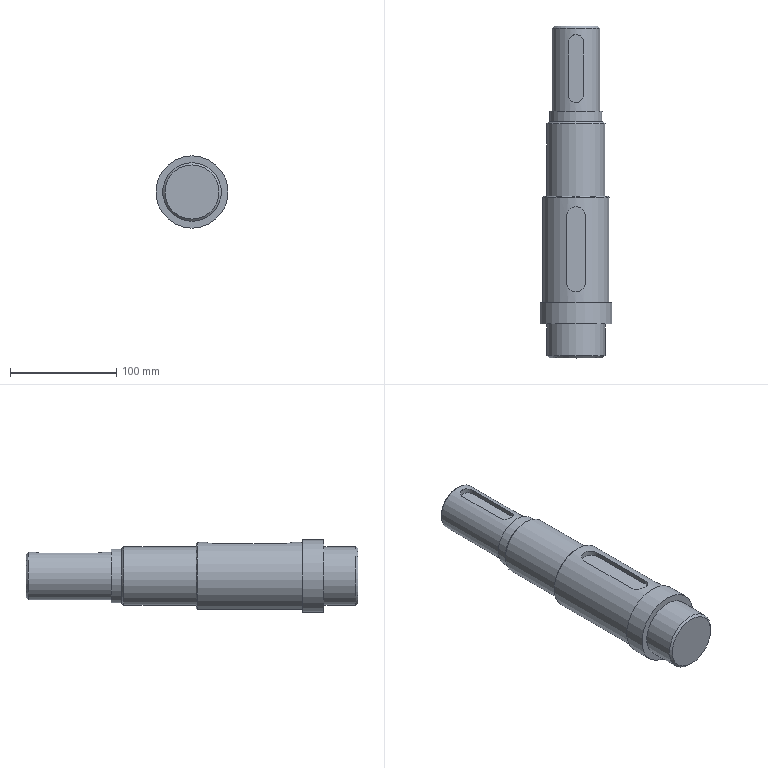Part | NX | features DATUM_CSYS 4, CHAMFER 3, SKETCH 3, DATUM_PLANE 2, EXTRUDE 2, SWP104 1 | 1 solid | 27 faces | box 68 x 312 x 68 mm | volume 761578 mm3 | plane 13 | cylinder 10 | cone 4 | commonest cylinder face diameters 14 x2 18 x2 55 x2 45 x1 50 x1 63 x1
STEP:
#1=CARTESIAN_POINT('',(0.,310.,22.5));
#2=VERTEX_POINT('',#1);
#3=CARTESIAN_POINT('',(0.,310.,0.));
#4=DIRECTION('',(0.,1.,0.));
#5=DIRECTION('',(0.,0.,1.));
#6=AXIS2_PLACEMENT_3D('',#3,#4,#5);
#7=CIRCLE('',#6,22.5);
#8=EDGE_CURVE('',#2,#2,#7,.F.);
#9=ORIENTED_EDGE('',*,*,#8,.T.);
#10=EDGE_LOOP('',(#9));
#11=FACE_BOUND('',#10,.T.);
#12=CARTESIAN_POINT('',(0.,232.,22.5));
#13=VERTEX_POINT('',#12);
#14=CARTESIAN_POINT('',(0.,232.,0.));
#15=DIRECTION('',(0.,1.,0.));
#16=DIRECTION('',(0.,0.,1.));
#17=AXIS2_PLACEMENT_3D('',#14,#15,#16);
#18=CIRCLE('',#17,22.5);
#19=EDGE_CURVE('',#13,#13,#18,.T.);
#20=ORIENTED_EDGE('',*,*,#19,.T.);
#21=EDGE_LOOP('',(#20));
#22=FACE_BOUND('',#21,.T.);
#23=CARTESIAN_POINT('',(7.,297.,21.383));
#24=VERTEX_POINT('',#23);
#25=CARTESIAN_POINT('',(7.,247.,21.383));
#26=VERTEX_POINT('',#25);
#27=CARTESIAN_POINT('',(7.,0.,21.383));
#28=DIRECTION('',(0.,1.,0.));
#29=VECTOR('',#28,1000.);
#30=LINE('',#27,#29);
#31=EDGE_CURVE('',#24,#26,#30,.F.);
#32=ORIENTED_EDGE('',*,*,#31,.T.);
#33=CARTESIAN_POINT('',(-7.,247.,21.383));
#34=VERTEX_POINT('',#33);
#35=CARTESIAN_POINT('',(7.,247.,21.383));
#36=CARTESIAN_POINT('',(7.,245.138,21.383));
#37=CARTESIAN_POINT('',(5.483,241.532,21.956));
#38=CARTESIAN_POINT('',(0.01146,239.235,22.772));
#39=CARTESIAN_POINT('',(-5.486,241.529,21.957));
#40=CARTESIAN_POINT('',(-7.,245.138,21.383));
#41=CARTESIAN_POINT('',(-7.,247.,21.383));
#42=B_SPLINE_CURVE_WITH_KNOTS('',3,(#35,#36,#37,#38,#39,#40,#41),.UNSPECIFIED.,.F.,.F.,(4,1,1,1,4),(0.,0.005504,0.01101,0.01651,0.02201),.UNSPECIFIED.);
#43=EDGE_CURVE('',#26,#34,#42,.T.);
#44=ORIENTED_EDGE('',*,*,#43,.T.);
#45=CARTESIAN_POINT('',(-7.,297.,21.383));
#46=VERTEX_POINT('',#45);
#47=CARTESIAN_POINT('',(-7.,0.,21.383));
#48=DIRECTION('',(0.,1.,0.));
#49=VECTOR('',#48,1000.);
#50=LINE('',#47,#49);
#51=EDGE_CURVE('',#34,#46,#50,.T.);
#52=ORIENTED_EDGE('',*,*,#51,.T.);
#53=CARTESIAN_POINT('',(-7.,297.,21.383));
#54=CARTESIAN_POINT('',(-7.,298.862,21.383));
#55=CARTESIAN_POINT('',(-5.483,302.468,21.956));
#56=CARTESIAN_POINT('',(-0.01146,304.765,22.772));
#57=CARTESIAN_POINT('',(5.486,302.471,21.957));
#58=CARTESIAN_POINT('',(7.,298.862,21.383));
#59=CARTESIAN_POINT('',(7.,297.,21.383));
#60=B_SPLINE_CURVE_WITH_KNOTS('',3,(#53,#54,#55,#56,#57,#58,#59),.UNSPECIFIED.,.F.,.F.,(4,1,1,1,4),(0.,0.005504,0.01101,0.01651,0.02201),.UNSPECIFIED.);
#61=EDGE_CURVE('',#46,#24,#60,.T.);
#62=ORIENTED_EDGE('',*,*,#61,.T.);
#63=EDGE_LOOP('',(#32,#44,#52,#62));
#64=FACE_BOUND('',#63,.T.);
#65=CARTESIAN_POINT('',(0.,0.,0.));
#66=DIRECTION('',(0.,1.,0.));
#67=DIRECTION('',(0.,0.,1.));
#68=AXIS2_PLACEMENT_3D('',#65,#66,#67);
#69=CYLINDRICAL_SURFACE('',#68,22.5);
#70=ADVANCED_FACE('',(#11,#22,#64),#69,.T.);
#71=CARTESIAN_POINT('',(0.,151.,31.5));
#72=VERTEX_POINT('',#71);
#73=CARTESIAN_POINT('',(0.,151.,0.));
#74=DIRECTION('',(0.,1.,0.));
#75=DIRECTION('',(0.,0.,1.));
#76=AXIS2_PLACEMENT_3D('',#73,#74,#75);
#77=CIRCLE('',#76,31.5);
#78=EDGE_CURVE('',#72,#72,#77,.F.);
#79=ORIENTED_EDGE('',*,*,#78,.T.);
#80=EDGE_LOOP('',(#79));
#81=FACE_BOUND('',#80,.T.);
#82=CARTESIAN_POINT('',(0.,52.,31.5));
#83=VERTEX_POINT('',#82);
#84=CARTESIAN_POINT('',(0.,52.,0.));
#85=DIRECTION('',(0.,1.,0.));
#86=DIRECTION('',(0.,0.,1.));
#87=AXIS2_PLACEMENT_3D('',#84,#85,#86);
#88=CIRCLE('',#87,31.5);
#89=EDGE_CURVE('',#83,#83,#88,.T.);
#90=ORIENTED_EDGE('',*,*,#89,.T.);
#91=EDGE_LOOP('',(#90));
#92=FACE_BOUND('',#91,.T.);
#93=CARTESIAN_POINT('',(9.,133.,30.187));
#94=VERTEX_POINT('',#93);
#95=CARTESIAN_POINT('',(9.,71.,30.187));
#96=VERTEX_POINT('',#95);
#97=CARTESIAN_POINT('',(9.,0.,30.187));
#98=DIRECTION('',(0.,1.,0.));
#99=VECTOR('',#98,1000.);
#100=LINE('',#97,#99);
#101=EDGE_CURVE('',#94,#96,#100,.F.);
#102=ORIENTED_EDGE('',*,*,#101,.T.);
#103=CARTESIAN_POINT('',(-9.,71.,30.187));
#104=VERTEX_POINT('',#103);
#105=CARTESIAN_POINT('',(9.,71.,30.187));
#106=CARTESIAN_POINT('',(9.,68.609,30.187));
#107=CARTESIAN_POINT('',(7.049,63.968,30.857));
#108=CARTESIAN_POINT('',(0.01381,61.017,31.821));
#109=CARTESIAN_POINT('',(-7.053,63.964,30.858));
#110=CARTESIAN_POINT('',(-9.,68.609,30.187));
#111=CARTESIAN_POINT('',(-9.,71.,30.187));
#112=B_SPLINE_CURVE_WITH_KNOTS('',3,(#105,#106,#107,#108,#109,#110,#111),.UNSPECIFIED.,.F.,.F.,(4,1,1,1,4),(0.,0.007069,0.01414,0.02121,0.02828),.UNSPECIFIED.);
#113=EDGE_CURVE('',#96,#104,#112,.T.);
#114=ORIENTED_EDGE('',*,*,#113,.T.);
#115=CARTESIAN_POINT('',(-9.,133.,30.187));
#116=VERTEX_POINT('',#115);
#117=CARTESIAN_POINT('',(-9.,0.,30.187));
#118=DIRECTION('',(0.,1.,0.));
#119=VECTOR('',#118,1000.);
#120=LINE('',#117,#119);
#121=EDGE_CURVE('',#104,#116,#120,.T.);
#122=ORIENTED_EDGE('',*,*,#121,.T.);
#123=CARTESIAN_POINT('',(-9.,133.,30.187));
#124=CARTESIAN_POINT('',(-9.,135.391,30.187));
#125=CARTESIAN_POINT('',(-7.049,140.032,30.857));
#126=CARTESIAN_POINT('',(-0.01381,142.983,31.821));
#127=CARTESIAN_POINT('',(7.053,140.036,30.858));
#128=CARTESIAN_POINT('',(9.,135.391,30.187));
#129=CARTESIAN_POINT('',(9.,133.,30.187));
#130=B_SPLINE_CURVE_WITH_KNOTS('',3,(#123,#124,#125,#126,#127,#128,#129),.UNSPECIFIED.,.F.,.F.,(4,1,1,1,4),(0.,0.007069,0.01414,0.02121,0.02828),.UNSPECIFIED.);
#131=EDGE_CURVE('',#116,#94,#130,.T.);
#132=ORIENTED_EDGE('',*,*,#131,.T.);
#133=EDGE_LOOP('',(#102,#114,#122,#132));
#134=FACE_BOUND('',#133,.T.);
#135=CARTESIAN_POINT('',(0.,0.,0.));
#136=DIRECTION('',(0.,1.,0.));
#137=DIRECTION('',(0.,0.,1.));
#138=AXIS2_PLACEMENT_3D('',#135,#136,#137);
#139=CYLINDRICAL_SURFACE('',#138,31.5);
#140=ADVANCED_FACE('',(#81,#92,#134),#139,.T.);
#141=CARTESIAN_POINT('',(0.,312.,20.5));
#142=VERTEX_POINT('',#141);
#143=CARTESIAN_POINT('',(0.,312.,0.));
#144=DIRECTION('',(0.,1.,0.));
#145=DIRECTION('',(0.,0.,1.));
#146=AXIS2_PLACEMENT_3D('',#143,#144,#145);
#147=CIRCLE('',#146,20.5);
#148=EDGE_CURVE('',#142,#142,#147,.T.);
#149=ORIENTED_EDGE('',*,*,#148,.T.);
#150=EDGE_LOOP('',(#149));
#151=FACE_BOUND('',#150,.T.);
#152=CARTESIAN_POINT('',(0.,312.,0.));
#153=DIRECTION('',(0.,1.,0.));
#154=DIRECTION('',(0.,0.,1.));
#155=AXIS2_PLACEMENT_3D('',#152,#153,#154);
#156=PLANE('',#155);
#157=ADVANCED_FACE('',(#151),#156,.T.);
#158=CARTESIAN_POINT('',(0.,232.,25.));
#159=VERTEX_POINT('',#158);
#160=CARTESIAN_POINT('',(0.,232.,0.));
#161=DIRECTION('',(0.,1.,0.));
#162=DIRECTION('',(0.,0.,1.));
#163=AXIS2_PLACEMENT_3D('',#160,#161,#162);
#164=CIRCLE('',#163,25.);
#165=EDGE_CURVE('',#159,#159,#164,.T.);
#166=ORIENTED_EDGE('',*,*,#165,.T.);
#167=EDGE_LOOP('',(#166));
#168=FACE_BOUND('',#167,.T.);
#169=ORIENTED_EDGE('',*,*,#19,.F.);
#170=EDGE_LOOP('',(#169));
#171=FACE_BOUND('',#170,.T.);
#172=CARTESIAN_POINT('',(0.,232.,22.5));
#173=DIRECTION('',(0.,1.,0.));
#174=DIRECTION('',(0.,0.,1.));
#175=AXIS2_PLACEMENT_3D('',#172,#173,#174);
#176=PLANE('',#175);
#177=ADVANCED_FACE('',(#168,#171),#176,.T.);
#178=CARTESIAN_POINT('',(0.,222.,25.));
#179=VERTEX_POINT('',#178);
#180=CARTESIAN_POINT('',(0.,222.,0.));
#181=DIRECTION('',(0.,1.,0.));
#182=DIRECTION('',(0.,0.,1.));
#183=AXIS2_PLACEMENT_3D('',#180,#181,#182);
#184=CIRCLE('',#183,25.);
#185=EDGE_CURVE('',#179,#179,#184,.T.);
#186=ORIENTED_EDGE('',*,*,#185,.T.);
#187=EDGE_LOOP('',(#186));
#188=FACE_BOUND('',#187,.T.);
#189=ORIENTED_EDGE('',*,*,#165,.F.);
#190=EDGE_LOOP('',(#189));
#191=FACE_BOUND('',#190,.T.);
#192=CARTESIAN_POINT('',(0.,0.,0.));
#193=DIRECTION('',(0.,1.,0.));
#194=DIRECTION('',(0.,0.,1.));
#195=AXIS2_PLACEMENT_3D('',#192,#193,#194);
#196=CYLINDRICAL_SURFACE('',#195,25.);
#197=ADVANCED_FACE('',(#188,#191),#196,.T.);
#198=CARTESIAN_POINT('',(0.,222.,25.5));
#199=VERTEX_POINT('',#198);
#200=CARTESIAN_POINT('',(0.,222.,0.));
#201=DIRECTION('',(0.,1.,0.));
#202=DIRECTION('',(0.,0.,1.));
#203=AXIS2_PLACEMENT_3D('',#200,#201,#202);
#204=CIRCLE('',#203,25.5);
#205=EDGE_CURVE('',#199,#199,#204,.T.);
#206=ORIENTED_EDGE('',*,*,#205,.T.);
#207=EDGE_LOOP('',(#206));
#208=FACE_BOUND('',#207,.T.);
#209=ORIENTED_EDGE('',*,*,#185,.F.);
#210=EDGE_LOOP('',(#209));
#211=FACE_BOUND('',#210,.T.);
#212=CARTESIAN_POINT('',(0.,222.,25.));
#213=DIRECTION('',(0.,1.,0.));
#214=DIRECTION('',(0.,0.,1.));
#215=AXIS2_PLACEMENT_3D('',#212,#213,#214);
#216=PLANE('',#215);
#217=ADVANCED_FACE('',(#208,#211),#216,.T.);
#218=CARTESIAN_POINT('',(0.,220.,27.5));
#219=VERTEX_POINT('',#218);
#220=CARTESIAN_POINT('',(0.,220.,0.));
#221=DIRECTION('',(0.,1.,0.));
#222=DIRECTION('',(0.,0.,1.));
#223=AXIS2_PLACEMENT_3D('',#220,#221,#222);
#224=CIRCLE('',#223,27.5);
#225=EDGE_CURVE('',#219,#219,#224,.F.);
#226=ORIENTED_EDGE('',*,*,#225,.T.);
#227=EDGE_LOOP('',(#226));
#228=FACE_BOUND('',#227,.T.);
#229=CARTESIAN_POINT('',(0.,152.,27.5));
#230=VERTEX_POINT('',#229);
#231=CARTESIAN_POINT('',(0.,152.,0.));
#232=DIRECTION('',(0.,1.,0.));
#233=DIRECTION('',(0.,0.,1.));
#234=AXIS2_PLACEMENT_3D('',#231,#232,#233);
#235=CIRCLE('',#234,27.5);
#236=EDGE_CURVE('',#230,#230,#235,.T.);
#237=ORIENTED_EDGE('',*,*,#236,.T.);
#238=EDGE_LOOP('',(#237));
#239=FACE_BOUND('',#238,.T.);
#240=CARTESIAN_POINT('',(0.,0.,0.));
#241=DIRECTION('',(0.,1.,0.));
#242=DIRECTION('',(0.,0.,1.));
#243=AXIS2_PLACEMENT_3D('',#240,#241,#242);
#244=CYLINDRICAL_SURFACE('',#243,27.5);
#245=ADVANCED_FACE('',(#228,#239),#244,.T.);
#246=CARTESIAN_POINT('',(0.,152.,30.5));
#247=VERTEX_POINT('',#246);
#248=CARTESIAN_POINT('',(0.,152.,0.));
#249=DIRECTION('',(0.,1.,0.));
#250=DIRECTION('',(0.,0.,1.));
#251=AXIS2_PLACEMENT_3D('',#248,#249,#250);
#252=CIRCLE('',#251,30.5);
#253=EDGE_CURVE('',#247,#247,#252,.T.);
#254=ORIENTED_EDGE('',*,*,#253,.T.);
#255=EDGE_LOOP('',(#254));
#256=FACE_BOUND('',#255,.T.);
#257=ORIENTED_EDGE('',*,*,#236,.F.);
#258=EDGE_LOOP('',(#257));
#259=FACE_BOUND('',#258,.T.);
#260=CARTESIAN_POINT('',(0.,152.,27.5));
#261=DIRECTION('',(0.,1.,0.));
#262=DIRECTION('',(0.,0.,1.));
#263=AXIS2_PLACEMENT_3D('',#260,#261,#262);
#264=PLANE('',#263);
#265=ADVANCED_FACE('',(#256,#259),#264,.T.);
#266=CARTESIAN_POINT('',(0.,52.,34.));
#267=VERTEX_POINT('',#266);
#268=CARTESIAN_POINT('',(0.,52.,0.));
#269=DIRECTION('',(0.,1.,0.));
#270=DIRECTION('',(0.,0.,1.));
#271=AXIS2_PLACEMENT_3D('',#268,#269,#270);
#272=CIRCLE('',#271,34.);
#273=EDGE_CURVE('',#267,#267,#272,.T.);
#274=ORIENTED_EDGE('',*,*,#273,.T.);
#275=EDGE_LOOP('',(#274));
#276=FACE_BOUND('',#275,.T.);
#277=ORIENTED_EDGE('',*,*,#89,.F.);
#278=EDGE_LOOP('',(#277));
#279=FACE_BOUND('',#278,.T.);
#280=CARTESIAN_POINT('',(0.,52.,31.5));
#281=DIRECTION('',(0.,1.,0.));
#282=DIRECTION('',(0.,0.,1.));
#283=AXIS2_PLACEMENT_3D('',#280,#281,#282);
#284=PLANE('',#283);
#285=ADVANCED_FACE('',(#276,#279),#284,.T.);
#286=CARTESIAN_POINT('',(0.,32.,34.));
#287=VERTEX_POINT('',#286);
#288=CARTESIAN_POINT('',(0.,32.,0.));
#289=DIRECTION('',(0.,1.,0.));
#290=DIRECTION('',(0.,0.,1.));
#291=AXIS2_PLACEMENT_3D('',#288,#289,#290);
#292=CIRCLE('',#291,34.);
#293=EDGE_CURVE('',#287,#287,#292,.T.);
#294=ORIENTED_EDGE('',*,*,#293,.T.);
#295=EDGE_LOOP('',(#294));
#296=FACE_BOUND('',#295,.T.);
#297=ORIENTED_EDGE('',*,*,#273,.F.);
#298=EDGE_LOOP('',(#297));
#299=FACE_BOUND('',#298,.T.);
#300=CARTESIAN_POINT('',(0.,0.,0.));
#301=DIRECTION('',(0.,1.,0.));
#302=DIRECTION('',(0.,0.,1.));
#303=AXIS2_PLACEMENT_3D('',#300,#301,#302);
#304=CYLINDRICAL_SURFACE('',#303,34.);
#305=ADVANCED_FACE('',(#296,#299),#304,.T.);
#306=CARTESIAN_POINT('',(0.,32.,27.5));
#307=VERTEX_POINT('',#306);
#308=CARTESIAN_POINT('',(0.,32.,0.));
#309=DIRECTION('',(0.,1.,0.));
#310=DIRECTION('',(0.,0.,1.));
#311=AXIS2_PLACEMENT_3D('',#308,#309,#310);
#312=CIRCLE('',#311,27.5);
#313=EDGE_CURVE('',#307,#307,#312,.T.);
#314=ORIENTED_EDGE('',*,*,#313,.T.);
#315=EDGE_LOOP('',(#314));
#316=FACE_BOUND('',#315,.T.);
#317=ORIENTED_EDGE('',*,*,#293,.F.);
#318=EDGE_LOOP('',(#317));
#319=FACE_BOUND('',#318,.T.);
#320=CARTESIAN_POINT('',(0.,32.,34.));
#321=DIRECTION('',(0.,-1.,0.));
#322=DIRECTION('',(0.,0.,-1.));
#323=AXIS2_PLACEMENT_3D('',#320,#321,#322);
#324=PLANE('',#323);
#325=ADVANCED_FACE('',(#316,#319),#324,.T.);
#326=CARTESIAN_POINT('',(0.,2.,-27.5));
#327=VERTEX_POINT('',#326);
#328=CARTESIAN_POINT('',(0.,2.,0.));
#329=DIRECTION('',(0.,-1.,0.));
#330=DIRECTION('',(0.,0.,-1.));
#331=AXIS2_PLACEMENT_3D('',#328,#329,#330);
#332=CIRCLE('',#331,27.5);
#333=EDGE_CURVE('',#327,#327,#332,.F.);
#334=ORIENTED_EDGE('',*,*,#333,.T.);
#335=EDGE_LOOP('',(#334));
#336=FACE_BOUND('',#335,.T.);
#337=ORIENTED_EDGE('',*,*,#313,.F.);
#338=EDGE_LOOP('',(#337));
#339=FACE_BOUND('',#338,.T.);
#340=CARTESIAN_POINT('',(0.,0.,0.));
#341=DIRECTION('',(0.,1.,0.));
#342=DIRECTION('',(0.,0.,1.));
#343=AXIS2_PLACEMENT_3D('',#340,#341,#342);
#344=CYLINDRICAL_SURFACE('',#343,27.5);
#345=ADVANCED_FACE('',(#336,#339),#344,.T.);
#346=CARTESIAN_POINT('',(0.,0.,-25.5));
#347=VERTEX_POINT('',#346);
#348=CARTESIAN_POINT('',(0.,0.,0.));
#349=DIRECTION('',(0.,-1.,0.));
#350=DIRECTION('',(0.,0.,-1.));
#351=AXIS2_PLACEMENT_3D('',#348,#349,#350);
#352=CIRCLE('',#351,25.5);
#353=EDGE_CURVE('',#347,#347,#352,.T.);
#354=ORIENTED_EDGE('',*,*,#353,.T.);
#355=EDGE_LOOP('',(#354));
#356=FACE_BOUND('',#355,.T.);
#357=CARTESIAN_POINT('',(0.,0.,27.5));
#358=DIRECTION('',(0.,-1.,0.));
#359=DIRECTION('',(0.,0.,-1.));
#360=AXIS2_PLACEMENT_3D('',#357,#358,#359);
#361=PLANE('',#360);
#362=ADVANCED_FACE('',(#356),#361,.T.);
#363=ORIENTED_EDGE('',*,*,#8,.F.);
#364=EDGE_LOOP('',(#363));
#365=FACE_BOUND('',#364,.T.);
#366=ORIENTED_EDGE('',*,*,#148,.F.);
#367=EDGE_LOOP('',(#366));
#368=FACE_BOUND('',#367,.T.);
#369=CARTESIAN_POINT('',(0.,312.,0.));
#370=DIRECTION('',(0.,-1.,0.));
#371=DIRECTION('',(0.,0.,-1.));
#372=AXIS2_PLACEMENT_3D('',#369,#370,#371);
#373=CONICAL_SURFACE('',#372,20.5,0.7854);
#374=ADVANCED_FACE('',(#365,#368),#373,.T.);
#375=ORIENTED_EDGE('',*,*,#353,.F.);
#376=EDGE_LOOP('',(#375));
#377=FACE_BOUND('',#376,.T.);
#378=ORIENTED_EDGE('',*,*,#333,.F.);
#379=EDGE_LOOP('',(#378));
#380=FACE_BOUND('',#379,.T.);
#381=CARTESIAN_POINT('',(0.,2.,0.));
#382=DIRECTION('',(0.,1.,0.));
#383=DIRECTION('',(0.,0.,1.));
#384=AXIS2_PLACEMENT_3D('',#381,#382,#383);
#385=CONICAL_SURFACE('',#384,27.5,0.7854);
#386=ADVANCED_FACE('',(#377,#380),#385,.T.);
#387=ORIENTED_EDGE('',*,*,#78,.F.);
#388=EDGE_LOOP('',(#387));
#389=FACE_BOUND('',#388,.T.);
#390=ORIENTED_EDGE('',*,*,#253,.F.);
#391=EDGE_LOOP('',(#390));
#392=FACE_BOUND('',#391,.T.);
#393=CARTESIAN_POINT('',(0.,152.,0.));
#394=DIRECTION('',(0.,-1.,0.));
#395=DIRECTION('',(0.,0.,-1.));
#396=AXIS2_PLACEMENT_3D('',#393,#394,#395);
#397=CONICAL_SURFACE('',#396,30.5,0.7854);
#398=ADVANCED_FACE('',(#389,#392),#397,.T.);
#399=CARTESIAN_POINT('',(-9.,71.,26.));
#400=VERTEX_POINT('',#399);
#401=CARTESIAN_POINT('',(-9.,71.,26.));
#402=DIRECTION('',(0.,0.,1.));
#403=VECTOR('',#402,1000.);
#404=LINE('',#401,#403);
#405=EDGE_CURVE('',#104,#400,#404,.F.);
#406=ORIENTED_EDGE('',*,*,#405,.T.);
#407=CARTESIAN_POINT('',(-9.,133.,26.));
#408=VERTEX_POINT('',#407);
#409=CARTESIAN_POINT('',(-9.,71.,26.));
#410=DIRECTION('',(0.,1.,0.));
#411=VECTOR('',#410,1000.);
#412=LINE('',#409,#411);
#413=EDGE_CURVE('',#408,#400,#412,.F.);
#414=ORIENTED_EDGE('',*,*,#413,.F.);
#415=CARTESIAN_POINT('',(-9.,133.,26.));
#416=DIRECTION('',(0.,0.,1.));
#417=VECTOR('',#416,1000.);
#418=LINE('',#415,#417);
#419=EDGE_CURVE('',#116,#408,#418,.F.);
#420=ORIENTED_EDGE('',*,*,#419,.F.);
#421=ORIENTED_EDGE('',*,*,#121,.F.);
#422=EDGE_LOOP('',(#406,#414,#420,#421));
#423=FACE_BOUND('',#422,.T.);
#424=CARTESIAN_POINT('',(-9.,71.,26.));
#425=DIRECTION('',(1.,0.,0.));
#426=DIRECTION('',(0.,1.,0.));
#427=AXIS2_PLACEMENT_3D('',#424,#425,#426);
#428=PLANE('',#427);
#429=ADVANCED_FACE('',(#423),#428,.T.);
#430=ORIENTED_EDGE('',*,*,#419,.T.);
#431=CARTESIAN_POINT('',(9.,133.,26.));
#432=VERTEX_POINT('',#431);
#433=CARTESIAN_POINT('',(0.,133.,26.));
#434=DIRECTION('',(0.,0.,-1.));
#435=DIRECTION('',(1.,0.,0.));
#436=AXIS2_PLACEMENT_3D('',#433,#434,#435);
#437=CIRCLE('',#436,9.);
#438=EDGE_CURVE('',#432,#408,#437,.F.);
#439=ORIENTED_EDGE('',*,*,#438,.F.);
#440=CARTESIAN_POINT('',(9.,133.,26.));
#441=DIRECTION('',(0.,0.,1.));
#442=VECTOR('',#441,1000.);
#443=LINE('',#440,#442);
#444=EDGE_CURVE('',#94,#432,#443,.F.);
#445=ORIENTED_EDGE('',*,*,#444,.F.);
#446=ORIENTED_EDGE('',*,*,#131,.F.);
#447=EDGE_LOOP('',(#430,#439,#445,#446));
#448=FACE_BOUND('',#447,.T.);
#449=CARTESIAN_POINT('',(0.,133.,26.));
#450=DIRECTION('',(0.,0.,1.));
#451=DIRECTION('',(1.,0.,0.));
#452=AXIS2_PLACEMENT_3D('',#449,#450,#451);
#453=CYLINDRICAL_SURFACE('',#452,9.);
#454=ADVANCED_FACE('',(#448),#453,.F.);
#455=ORIENTED_EDGE('',*,*,#444,.T.);
#456=CARTESIAN_POINT('',(9.,71.,26.));
#457=VERTEX_POINT('',#456);
#458=CARTESIAN_POINT('',(9.,133.,26.));
#459=DIRECTION('',(0.,-1.,0.));
#460=VECTOR('',#459,1000.);
#461=LINE('',#458,#460);
#462=EDGE_CURVE('',#457,#432,#461,.F.);
#463=ORIENTED_EDGE('',*,*,#462,.F.);
#464=CARTESIAN_POINT('',(9.,71.,26.));
#465=DIRECTION('',(0.,0.,1.));
#466=VECTOR('',#465,1000.);
#467=LINE('',#464,#466);
#468=EDGE_CURVE('',#96,#457,#467,.F.);
#469=ORIENTED_EDGE('',*,*,#468,.F.);
#470=ORIENTED_EDGE('',*,*,#101,.F.);
#471=EDGE_LOOP('',(#455,#463,#469,#470));
#472=FACE_BOUND('',#471,.T.);
#473=CARTESIAN_POINT('',(9.,133.,26.));
#474=DIRECTION('',(-1.,0.,0.));
#475=DIRECTION('',(0.,-1.,0.));
#476=AXIS2_PLACEMENT_3D('',#473,#474,#475);
#477=PLANE('',#476);
#478=ADVANCED_FACE('',(#472),#477,.T.);
#479=ORIENTED_EDGE('',*,*,#468,.T.);
#480=CARTESIAN_POINT('',(0.,71.,26.));
#481=DIRECTION('',(0.,0.,-1.));
#482=DIRECTION('',(1.,0.,0.));
#483=AXIS2_PLACEMENT_3D('',#480,#481,#482);
#484=CIRCLE('',#483,9.);
#485=EDGE_CURVE('',#400,#457,#484,.F.);
#486=ORIENTED_EDGE('',*,*,#485,.F.);
#487=ORIENTED_EDGE('',*,*,#405,.F.);
#488=ORIENTED_EDGE('',*,*,#113,.F.);
#489=EDGE_LOOP('',(#479,#486,#487,#488));
#490=FACE_BOUND('',#489,.T.);
#491=CARTESIAN_POINT('',(0.,71.,26.));
#492=DIRECTION('',(0.,0.,1.));
#493=DIRECTION('',(1.,0.,0.));
#494=AXIS2_PLACEMENT_3D('',#491,#492,#493);
#495=CYLINDRICAL_SURFACE('',#494,9.);
#496=ADVANCED_FACE('',(#490),#495,.F.);
#497=ORIENTED_EDGE('',*,*,#413,.T.);
#498=ORIENTED_EDGE('',*,*,#485,.T.);
#499=ORIENTED_EDGE('',*,*,#462,.T.);
#500=ORIENTED_EDGE('',*,*,#438,.T.);
#501=EDGE_LOOP('',(#497,#498,#499,#500));
#502=FACE_BOUND('',#501,.T.);
#503=CARTESIAN_POINT('',(0.,133.,26.));
#504=DIRECTION('',(0.,0.,-1.));
#505=DIRECTION('',(-1.,0.,0.));
#506=AXIS2_PLACEMENT_3D('',#503,#504,#505);
#507=PLANE('',#506);
#508=ADVANCED_FACE('',(#502),#507,.F.);
#509=CARTESIAN_POINT('',(-7.,247.,17.5));
#510=VERTEX_POINT('',#509);
#511=CARTESIAN_POINT('',(-7.,247.,17.5));
#512=DIRECTION('',(0.,0.,1.));
#513=VECTOR('',#512,1000.);
#514=LINE('',#511,#513);
#515=EDGE_CURVE('',#34,#510,#514,.F.);
#516=ORIENTED_EDGE('',*,*,#515,.T.);
#517=CARTESIAN_POINT('',(-7.,297.,17.5));
#518=VERTEX_POINT('',#517);
#519=CARTESIAN_POINT('',(-7.,247.,17.5));
#520=DIRECTION('',(0.,1.,0.));
#521=VECTOR('',#520,1000.);
#522=LINE('',#519,#521);
#523=EDGE_CURVE('',#518,#510,#522,.F.);
#524=ORIENTED_EDGE('',*,*,#523,.F.);
#525=CARTESIAN_POINT('',(-7.,297.,17.5));
#526=DIRECTION('',(0.,0.,1.));
#527=VECTOR('',#526,1000.);
#528=LINE('',#525,#527);
#529=EDGE_CURVE('',#46,#518,#528,.F.);
#530=ORIENTED_EDGE('',*,*,#529,.F.);
#531=ORIENTED_EDGE('',*,*,#51,.F.);
#532=EDGE_LOOP('',(#516,#524,#530,#531));
#533=FACE_BOUND('',#532,.T.);
#534=CARTESIAN_POINT('',(-7.,247.,17.5));
#535=DIRECTION('',(1.,0.,0.));
#536=DIRECTION('',(0.,0.,-1.));
#537=AXIS2_PLACEMENT_3D('',#534,#535,#536);
#538=PLANE('',#537);
#539=ADVANCED_FACE('',(#533),#538,.T.);
#540=ORIENTED_EDGE('',*,*,#529,.T.);
#541=CARTESIAN_POINT('',(7.,297.,17.5));
#542=VERTEX_POINT('',#541);
#543=CARTESIAN_POINT('',(0.,297.,17.5));
#544=DIRECTION('',(0.,0.,-1.));
#545=DIRECTION('',(1.,0.,0.));
#546=AXIS2_PLACEMENT_3D('',#543,#544,#545);
#547=CIRCLE('',#546,7.);
#548=EDGE_CURVE('',#542,#518,#547,.F.);
#549=ORIENTED_EDGE('',*,*,#548,.F.);
#550=CARTESIAN_POINT('',(7.,297.,17.5));
#551=DIRECTION('',(0.,0.,1.));
#552=VECTOR('',#551,1000.);
#553=LINE('',#550,#552);
#554=EDGE_CURVE('',#24,#542,#553,.F.);
#555=ORIENTED_EDGE('',*,*,#554,.F.);
#556=ORIENTED_EDGE('',*,*,#61,.F.);
#557=EDGE_LOOP('',(#540,#549,#555,#556));
#558=FACE_BOUND('',#557,.T.);
#559=CARTESIAN_POINT('',(0.,297.,17.5));
#560=DIRECTION('',(0.,0.,1.));
#561=DIRECTION('',(1.,0.,0.));
#562=AXIS2_PLACEMENT_3D('',#559,#560,#561);
#563=CYLINDRICAL_SURFACE('',#562,7.);
#564=ADVANCED_FACE('',(#558),#563,.F.);
#565=ORIENTED_EDGE('',*,*,#554,.T.);
#566=CARTESIAN_POINT('',(7.,247.,17.5));
#567=VERTEX_POINT('',#566);
#568=CARTESIAN_POINT('',(7.,297.,17.5));
#569=DIRECTION('',(0.,-1.,0.));
#570=VECTOR('',#569,1000.);
#571=LINE('',#568,#570);
#572=EDGE_CURVE('',#567,#542,#571,.F.);
#573=ORIENTED_EDGE('',*,*,#572,.F.);
#574=CARTESIAN_POINT('',(7.,247.,17.5));
#575=DIRECTION('',(0.,0.,1.));
#576=VECTOR('',#575,1000.);
#577=LINE('',#574,#576);
#578=EDGE_CURVE('',#26,#567,#577,.F.);
#579=ORIENTED_EDGE('',*,*,#578,.F.);
#580=ORIENTED_EDGE('',*,*,#31,.F.);
#581=EDGE_LOOP('',(#565,#573,#579,#580));
#582=FACE_BOUND('',#581,.T.);
#583=CARTESIAN_POINT('',(7.,297.,17.5));
#584=DIRECTION('',(-1.,0.,0.));
#585=DIRECTION('',(0.,0.,1.));
#586=AXIS2_PLACEMENT_3D('',#583,#584,#585);
#587=PLANE('',#586);
#588=ADVANCED_FACE('',(#582),#587,.T.);
#589=ORIENTED_EDGE('',*,*,#578,.T.);
#590=CARTESIAN_POINT('',(0.,247.,17.5));
#591=DIRECTION('',(0.,0.,-1.));
#592=DIRECTION('',(1.,0.,0.));
#593=AXIS2_PLACEMENT_3D('',#590,#591,#592);
#594=CIRCLE('',#593,7.);
#595=EDGE_CURVE('',#510,#567,#594,.F.);
#596=ORIENTED_EDGE('',*,*,#595,.F.);
#597=ORIENTED_EDGE('',*,*,#515,.F.);
#598=ORIENTED_EDGE('',*,*,#43,.F.);
#599=EDGE_LOOP('',(#589,#596,#597,#598));
#600=FACE_BOUND('',#599,.T.);
#601=CARTESIAN_POINT('',(0.,247.,17.5));
#602=DIRECTION('',(0.,0.,1.));
#603=DIRECTION('',(1.,0.,0.));
#604=AXIS2_PLACEMENT_3D('',#601,#602,#603);
#605=CYLINDRICAL_SURFACE('',#604,7.);
#606=ADVANCED_FACE('',(#600),#605,.F.);
#607=ORIENTED_EDGE('',*,*,#523,.T.);
#608=ORIENTED_EDGE('',*,*,#595,.T.);
#609=ORIENTED_EDGE('',*,*,#572,.T.);
#610=ORIENTED_EDGE('',*,*,#548,.T.);
#611=EDGE_LOOP('',(#607,#608,#609,#610));
#612=FACE_BOUND('',#611,.T.);
#613=CARTESIAN_POINT('',(0.,297.,17.5));
#614=DIRECTION('',(0.,0.,-1.));
#615=DIRECTION('',(-1.,0.,0.));
#616=AXIS2_PLACEMENT_3D('',#613,#614,#615);
#617=PLANE('',#616);
#618=ADVANCED_FACE('',(#612),#617,.F.);
#619=ORIENTED_EDGE('',*,*,#225,.F.);
#620=EDGE_LOOP('',(#619));
#621=FACE_BOUND('',#620,.T.);
#622=ORIENTED_EDGE('',*,*,#205,.F.);
#623=EDGE_LOOP('',(#622));
#624=FACE_BOUND('',#623,.T.);
#625=CARTESIAN_POINT('',(0.,222.,0.));
#626=DIRECTION('',(0.,-1.,0.));
#627=DIRECTION('',(0.,0.,-1.));
#628=AXIS2_PLACEMENT_3D('',#625,#626,#627);
#629=CONICAL_SURFACE('',#628,25.5,0.7854);
#630=ADVANCED_FACE('',(#621,#624),#629,.T.);
#631=CLOSED_SHELL('',(#70,#140,#157,#177,#197,#217,#245,#265,#285,#305,#325,#345,#362,#374,#386,#398,#429,#454,#478,#496,#508,#539,#564,#588,#606,#618,#630));
#632=MANIFOLD_SOLID_BREP('',#631);
#633=(LENGTH_UNIT()NAMED_UNIT(*)SI_UNIT(.MILLI.,.METRE.));
#634=UNCERTAINTY_MEASURE_WITH_UNIT(LENGTH_MEASURE(0.0508),#633,'','');
#635=(NAMED_UNIT(*)PLANE_ANGLE_UNIT()SI_UNIT($,.RADIAN.));
#636=(NAMED_UNIT(*)SI_UNIT($,.STERADIAN.)SOLID_ANGLE_UNIT());
#637=(GEOMETRIC_REPRESENTATION_CONTEXT(3)GLOBAL_UNCERTAINTY_ASSIGNED_CONTEXT((#634))GLOBAL_UNIT_ASSIGNED_CONTEXT((#633,#635,#636))REPRESENTATION_CONTEXT('',''));
#638=ADVANCED_BREP_SHAPE_REPRESENTATION('',(#632),#637);